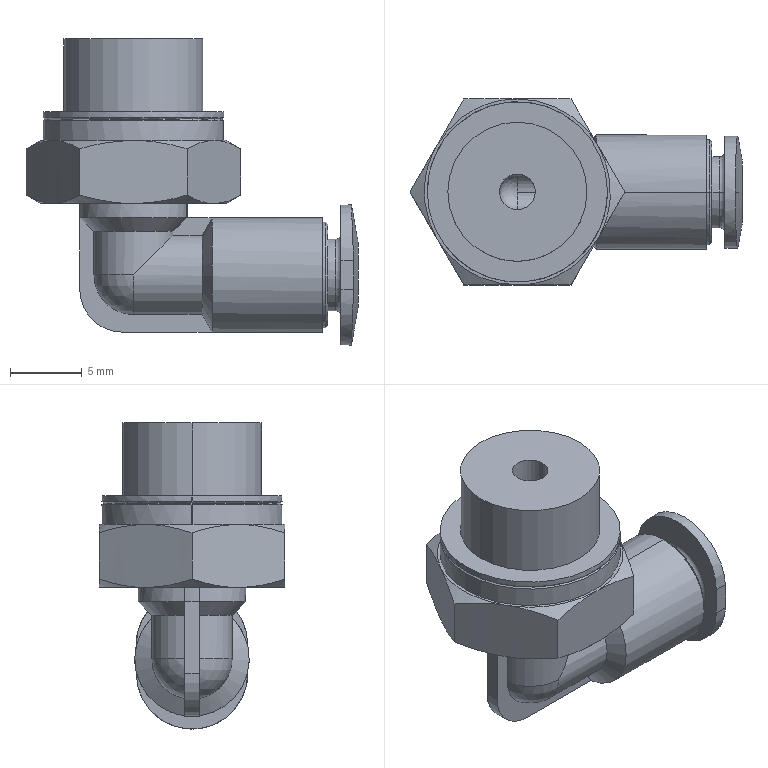Part | SolidWorks | features ICE 10, Fillet 2, BaseBody 1, Chamfer 1, HoleWzd 1, RevCut 1 | 1 solid | 104 faces | box 23.206 x 13 x 21.4 mm | volume 1816 mm3 | cylinder 44 | plane 29 | cone 24 | torus 4 | sphere 3 | commonest cylinder face diameters 12.6 x12 2.5 x4 5.6 x4 7.492 x4 8 x4 9.728 x4